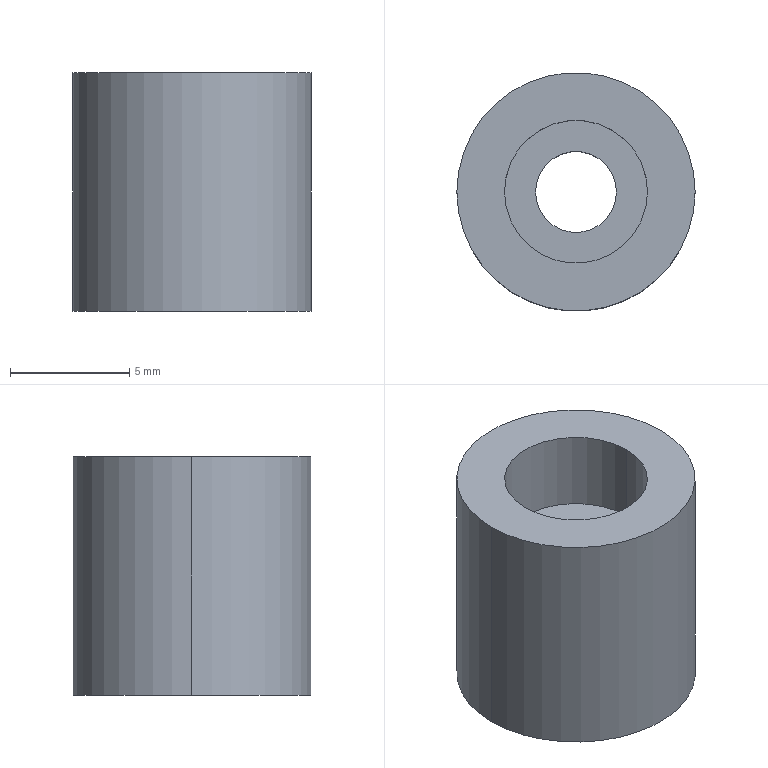Part | NX | features BREP 1 | 1 solid | 9 faces | box 10 x 10 x 10 mm | volume 629.343 mm3 | cylinder 6 | plane 3 | commonest cylinder face diameters 3.4 x2 6 x2 10 x2
STEP:
#1=CARTESIAN_POINT('',(-3.,0.,10.));
#2=VERTEX_POINT('',#1);
#3=CARTESIAN_POINT('',(-3.,0.,6.6));
#4=VERTEX_POINT('',#3);
#5=CARTESIAN_POINT('',(-3.,0.,10.));
#6=DIRECTION('',(0.,0.,1.));
#7=VECTOR('',#6,1000.);
#8=LINE('',#5,#7);
#9=EDGE_CURVE('',#2,#4,#8,.F.);
#10=ORIENTED_EDGE('',*,*,#9,.T.);
#11=CARTESIAN_POINT('',(3.,0.,6.6));
#12=VERTEX_POINT('',#11);
#13=CARTESIAN_POINT('',(0.,0.,6.6));
#14=DIRECTION('',(0.,0.,1.));
#15=DIRECTION('',(1.,0.,0.));
#16=AXIS2_PLACEMENT_3D('',#13,#14,#15);
#17=CIRCLE('',#16,3.);
#18=EDGE_CURVE('',#12,#4,#17,.T.);
#19=ORIENTED_EDGE('',*,*,#18,.F.);
#20=CARTESIAN_POINT('',(3.,0.,10.));
#21=VERTEX_POINT('',#20);
#22=CARTESIAN_POINT('',(3.,0.,10.));
#23=DIRECTION('',(0.,0.,1.));
#24=VECTOR('',#23,1000.);
#25=LINE('',#22,#24);
#26=EDGE_CURVE('',#21,#12,#25,.F.);
#27=ORIENTED_EDGE('',*,*,#26,.F.);
#28=CARTESIAN_POINT('',(0.,0.,10.));
#29=DIRECTION('',(0.,0.,1.));
#30=DIRECTION('',(1.,0.,0.));
#31=AXIS2_PLACEMENT_3D('',#28,#29,#30);
#32=CIRCLE('',#31,3.);
#33=EDGE_CURVE('',#21,#2,#32,.T.);
#34=ORIENTED_EDGE('',*,*,#33,.T.);
#35=EDGE_LOOP('',(#10,#19,#27,#34));
#36=FACE_BOUND('',#35,.T.);
#37=CARTESIAN_POINT('',(0.,0.,10.));
#38=DIRECTION('',(0.,0.,1.));
#39=DIRECTION('',(1.,0.,0.));
#40=AXIS2_PLACEMENT_3D('',#37,#38,#39);
#41=CYLINDRICAL_SURFACE('',#40,3.);
#42=ADVANCED_FACE('',(#36),#41,.F.);
#43=ORIENTED_EDGE('',*,*,#18,.T.);
#44=CARTESIAN_POINT('',(0.,0.,6.6));
#45=DIRECTION('',(0.,0.,1.));
#46=DIRECTION('',(1.,0.,0.));
#47=AXIS2_PLACEMENT_3D('',#44,#45,#46);
#48=CIRCLE('',#47,3.);
#49=EDGE_CURVE('',#4,#12,#48,.T.);
#50=ORIENTED_EDGE('',*,*,#49,.T.);
#51=EDGE_LOOP('',(#43,#50));
#52=FACE_BOUND('',#51,.T.);
#53=CARTESIAN_POINT('',(1.7,0.,6.6));
#54=VERTEX_POINT('',#53);
#55=CARTESIAN_POINT('',(-1.7,0.,6.6));
#56=VERTEX_POINT('',#55);
#57=CARTESIAN_POINT('',(0.,0.,6.6));
#58=DIRECTION('',(0.,0.,1.));
#59=DIRECTION('',(1.,0.,0.));
#60=AXIS2_PLACEMENT_3D('',#57,#58,#59);
#61=CIRCLE('',#60,1.7);
#62=EDGE_CURVE('',#54,#56,#61,.T.);
#63=ORIENTED_EDGE('',*,*,#62,.F.);
#64=CARTESIAN_POINT('',(0.,0.,6.6));
#65=DIRECTION('',(0.,0.,1.));
#66=DIRECTION('',(1.,0.,0.));
#67=AXIS2_PLACEMENT_3D('',#64,#65,#66);
#68=CIRCLE('',#67,1.7);
#69=EDGE_CURVE('',#56,#54,#68,.T.);
#70=ORIENTED_EDGE('',*,*,#69,.F.);
#71=EDGE_LOOP('',(#63,#70));
#72=FACE_BOUND('',#71,.T.);
#73=CARTESIAN_POINT('',(1.7,0.,6.6));
#74=DIRECTION('',(0.,0.,-1.));
#75=DIRECTION('',(-1.,0.,0.));
#76=AXIS2_PLACEMENT_3D('',#73,#74,#75);
#77=PLANE('',#76);
#78=ADVANCED_FACE('',(#52,#72),#77,.F.);
#79=CARTESIAN_POINT('',(-1.7,0.,0.));
#80=VERTEX_POINT('',#79);
#81=CARTESIAN_POINT('',(-1.7,0.,10.));
#82=DIRECTION('',(0.,0.,1.));
#83=VECTOR('',#82,1000.);
#84=LINE('',#81,#83);
#85=EDGE_CURVE('',#56,#80,#84,.F.);
#86=ORIENTED_EDGE('',*,*,#85,.T.);
#87=CARTESIAN_POINT('',(1.7,0.,0.));
#88=VERTEX_POINT('',#87);
#89=CARTESIAN_POINT('',(0.,0.,0.));
#90=DIRECTION('',(0.,0.,1.));
#91=DIRECTION('',(1.,0.,0.));
#92=AXIS2_PLACEMENT_3D('',#89,#90,#91);
#93=CIRCLE('',#92,1.7);
#94=EDGE_CURVE('',#88,#80,#93,.T.);
#95=ORIENTED_EDGE('',*,*,#94,.F.);
#96=CARTESIAN_POINT('',(1.7,0.,10.));
#97=DIRECTION('',(0.,0.,1.));
#98=VECTOR('',#97,1000.);
#99=LINE('',#96,#98);
#100=EDGE_CURVE('',#54,#88,#99,.F.);
#101=ORIENTED_EDGE('',*,*,#100,.F.);
#102=ORIENTED_EDGE('',*,*,#62,.T.);
#103=EDGE_LOOP('',(#86,#95,#101,#102));
#104=FACE_BOUND('',#103,.T.);
#105=CARTESIAN_POINT('',(0.,0.,10.));
#106=DIRECTION('',(0.,0.,1.));
#107=DIRECTION('',(1.,0.,0.));
#108=AXIS2_PLACEMENT_3D('',#105,#106,#107);
#109=CYLINDRICAL_SURFACE('',#108,1.7);
#110=ADVANCED_FACE('',(#104),#109,.F.);
#111=CARTESIAN_POINT('',(-5.,0.,0.));
#112=VERTEX_POINT('',#111);
#113=CARTESIAN_POINT('',(5.,0.,0.));
#114=VERTEX_POINT('',#113);
#115=CARTESIAN_POINT('',(0.,0.,0.));
#116=DIRECTION('',(0.,0.,1.));
#117=DIRECTION('',(1.,0.,0.));
#118=AXIS2_PLACEMENT_3D('',#115,#116,#117);
#119=CIRCLE('',#118,5.);
#120=EDGE_CURVE('',#112,#114,#119,.T.);
#121=ORIENTED_EDGE('',*,*,#120,.F.);
#122=CARTESIAN_POINT('',(0.,0.,0.));
#123=DIRECTION('',(0.,0.,1.));
#124=DIRECTION('',(1.,0.,0.));
#125=AXIS2_PLACEMENT_3D('',#122,#123,#124);
#126=CIRCLE('',#125,5.);
#127=EDGE_CURVE('',#114,#112,#126,.T.);
#128=ORIENTED_EDGE('',*,*,#127,.F.);
#129=EDGE_LOOP('',(#121,#128));
#130=FACE_BOUND('',#129,.T.);
#131=ORIENTED_EDGE('',*,*,#94,.T.);
#132=CARTESIAN_POINT('',(0.,0.,0.));
#133=DIRECTION('',(0.,0.,1.));
#134=DIRECTION('',(1.,0.,0.));
#135=AXIS2_PLACEMENT_3D('',#132,#133,#134);
#136=CIRCLE('',#135,1.7);
#137=EDGE_CURVE('',#80,#88,#136,.T.);
#138=ORIENTED_EDGE('',*,*,#137,.T.);
#139=EDGE_LOOP('',(#131,#138));
#140=FACE_BOUND('',#139,.T.);
#141=CARTESIAN_POINT('',(0.,0.,0.));
#142=DIRECTION('',(0.,0.,1.));
#143=DIRECTION('',(1.,0.,0.));
#144=AXIS2_PLACEMENT_3D('',#141,#142,#143);
#145=PLANE('',#144);
#146=ADVANCED_FACE('',(#130,#140),#145,.F.);
#147=CARTESIAN_POINT('',(-5.,0.,10.));
#148=VERTEX_POINT('',#147);
#149=CARTESIAN_POINT('',(5.,0.,10.));
#150=VERTEX_POINT('',#149);
#151=CARTESIAN_POINT('',(0.,0.,10.));
#152=DIRECTION('',(0.,0.,1.));
#153=DIRECTION('',(1.,0.,0.));
#154=AXIS2_PLACEMENT_3D('',#151,#152,#153);
#155=CIRCLE('',#154,5.);
#156=EDGE_CURVE('',#148,#150,#155,.T.);
#157=ORIENTED_EDGE('',*,*,#156,.T.);
#158=CARTESIAN_POINT('',(0.,0.,10.));
#159=DIRECTION('',(0.,0.,1.));
#160=DIRECTION('',(1.,0.,0.));
#161=AXIS2_PLACEMENT_3D('',#158,#159,#160);
#162=CIRCLE('',#161,5.);
#163=EDGE_CURVE('',#150,#148,#162,.T.);
#164=ORIENTED_EDGE('',*,*,#163,.T.);
#165=EDGE_LOOP('',(#157,#164));
#166=FACE_BOUND('',#165,.T.);
#167=ORIENTED_EDGE('',*,*,#33,.F.);
#168=CARTESIAN_POINT('',(0.,0.,10.));
#169=DIRECTION('',(0.,0.,1.));
#170=DIRECTION('',(1.,0.,0.));
#171=AXIS2_PLACEMENT_3D('',#168,#169,#170);
#172=CIRCLE('',#171,3.);
#173=EDGE_CURVE('',#2,#21,#172,.T.);
#174=ORIENTED_EDGE('',*,*,#173,.F.);
#175=EDGE_LOOP('',(#167,#174));
#176=FACE_BOUND('',#175,.T.);
#177=CARTESIAN_POINT('',(0.,0.,10.));
#178=DIRECTION('',(0.,0.,1.));
#179=DIRECTION('',(1.,0.,0.));
#180=AXIS2_PLACEMENT_3D('',#177,#178,#179);
#181=PLANE('',#180);
#182=ADVANCED_FACE('',(#166,#176),#181,.T.);
#183=CARTESIAN_POINT('',(5.,0.,10.));
#184=DIRECTION('',(0.,0.,-1.));
#185=VECTOR('',#184,1000.);
#186=LINE('',#183,#185);
#187=EDGE_CURVE('',#150,#114,#186,.T.);
#188=ORIENTED_EDGE('',*,*,#187,.F.);
#189=ORIENTED_EDGE('',*,*,#156,.F.);
#190=CARTESIAN_POINT('',(-5.,0.,10.));
#191=DIRECTION('',(0.,0.,-1.));
#192=VECTOR('',#191,1000.);
#193=LINE('',#190,#192);
#194=EDGE_CURVE('',#148,#112,#193,.T.);
#195=ORIENTED_EDGE('',*,*,#194,.T.);
#196=ORIENTED_EDGE('',*,*,#120,.T.);
#197=EDGE_LOOP('',(#188,#189,#195,#196));
#198=FACE_BOUND('',#197,.T.);
#199=CARTESIAN_POINT('',(0.,0.,10.));
#200=DIRECTION('',(0.,0.,-1.));
#201=DIRECTION('',(-1.,0.,0.));
#202=AXIS2_PLACEMENT_3D('',#199,#200,#201);
#203=CYLINDRICAL_SURFACE('',#202,5.);
#204=ADVANCED_FACE('',(#198),#203,.T.);
#205=ORIENTED_EDGE('',*,*,#163,.F.);
#206=ORIENTED_EDGE('',*,*,#187,.T.);
#207=ORIENTED_EDGE('',*,*,#127,.T.);
#208=ORIENTED_EDGE('',*,*,#194,.F.);
#209=EDGE_LOOP('',(#205,#206,#207,#208));
#210=FACE_BOUND('',#209,.T.);
#211=CARTESIAN_POINT('',(0.,0.,10.));
#212=DIRECTION('',(0.,0.,-1.));
#213=DIRECTION('',(-1.,0.,0.));
#214=AXIS2_PLACEMENT_3D('',#211,#212,#213);
#215=CYLINDRICAL_SURFACE('',#214,5.);
#216=ADVANCED_FACE('',(#210),#215,.T.);
#217=ORIENTED_EDGE('',*,*,#137,.F.);
#218=ORIENTED_EDGE('',*,*,#85,.F.);
#219=ORIENTED_EDGE('',*,*,#69,.T.);
#220=ORIENTED_EDGE('',*,*,#100,.T.);
#221=EDGE_LOOP('',(#217,#218,#219,#220));
#222=FACE_BOUND('',#221,.T.);
#223=CARTESIAN_POINT('',(0.,0.,10.));
#224=DIRECTION('',(0.,0.,1.));
#225=DIRECTION('',(1.,0.,0.));
#226=AXIS2_PLACEMENT_3D('',#223,#224,#225);
#227=CYLINDRICAL_SURFACE('',#226,1.7);
#228=ADVANCED_FACE('',(#222),#227,.F.);
#229=ORIENTED_EDGE('',*,*,#49,.F.);
#230=ORIENTED_EDGE('',*,*,#9,.F.);
#231=ORIENTED_EDGE('',*,*,#173,.T.);
#232=ORIENTED_EDGE('',*,*,#26,.T.);
#233=EDGE_LOOP('',(#229,#230,#231,#232));
#234=FACE_BOUND('',#233,.T.);
#235=CARTESIAN_POINT('',(0.,0.,10.));
#236=DIRECTION('',(0.,0.,1.));
#237=DIRECTION('',(1.,0.,0.));
#238=AXIS2_PLACEMENT_3D('',#235,#236,#237);
#239=CYLINDRICAL_SURFACE('',#238,3.);
#240=ADVANCED_FACE('',(#234),#239,.F.);
#241=CLOSED_SHELL('',(#42,#78,#110,#146,#182,#204,#216,#228,#240));
#242=MANIFOLD_SOLID_BREP('',#241);
#243=(LENGTH_UNIT()NAMED_UNIT(*)SI_UNIT(.MILLI.,.METRE.));
#244=UNCERTAINTY_MEASURE_WITH_UNIT(LENGTH_MEASURE(0.00001),#243,'','');
#245=(NAMED_UNIT(*)PLANE_ANGLE_UNIT()SI_UNIT($,.RADIAN.));
#246=(NAMED_UNIT(*)SI_UNIT($,.STERADIAN.)SOLID_ANGLE_UNIT());
#247=(GEOMETRIC_REPRESENTATION_CONTEXT(3)GLOBAL_UNCERTAINTY_ASSIGNED_CONTEXT((#244))GLOBAL_UNIT_ASSIGNED_CONTEXT((#243,#245,#246))REPRESENTATION_CONTEXT('',''));
#248=ADVANCED_BREP_SHAPE_REPRESENTATION('',(#242),#247);